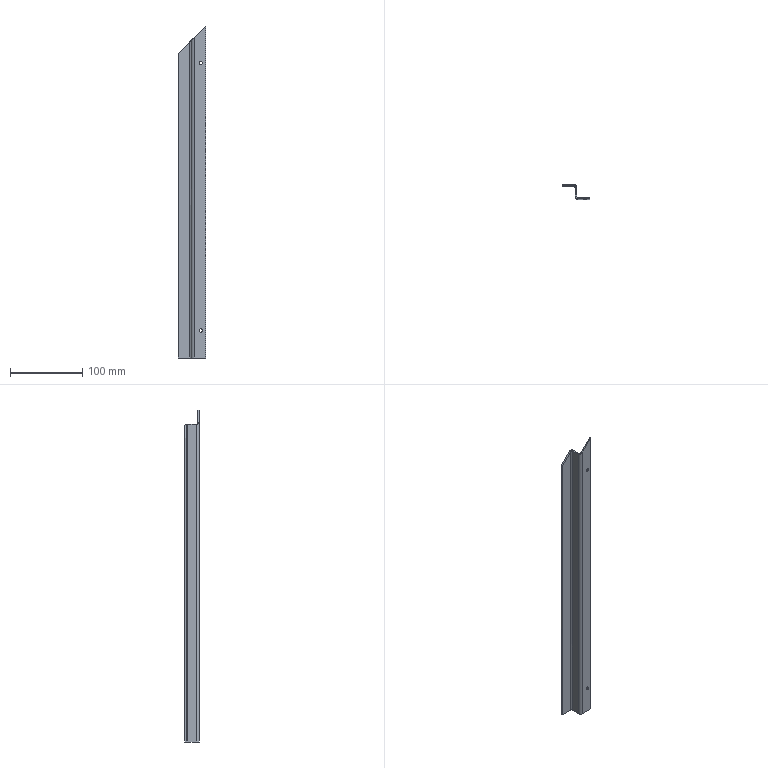Part | STEP file | SYL_0392D6J1SYL0380DJ10-1205588 | 1 solid | 26 faces | box 38 x 20 x 458 mm | volume 46808 mm3 | plane 16 | cylinder 8 | spline 2 | commonest cylinder face diameters 4.5 x4 4 x2 8 x2
STEP:
#1=CARTESIAN_POINT('',(11.,-20.,-193.25));
#2=VERTEX_POINT('',#1);
#3=CARTESIAN_POINT('',(11.,-18.,-193.25));
#4=VERTEX_POINT('',#3);
#5=CARTESIAN_POINT('',(11.,-18.,-193.25));
#6=DIRECTION('',(0.,1.,0.));
#7=VECTOR('',#6,1000.);
#8=LINE('',#5,#7);
#9=EDGE_CURVE('',#2,#4,#8,.T.);
#10=ORIENTED_EDGE('',*,*,#9,.F.);
#11=CARTESIAN_POINT('',(11.,-20.,-188.75));
#12=VERTEX_POINT('',#11);
#13=CARTESIAN_POINT('',(11.,-20.,-191.));
#14=DIRECTION('',(0.,-1.,0.));
#15=DIRECTION('',(0.,0.,-1.));
#16=AXIS2_PLACEMENT_3D('',#13,#14,#15);
#17=CIRCLE('',#16,2.25);
#18=EDGE_CURVE('',#2,#12,#17,.T.);
#19=ORIENTED_EDGE('',*,*,#18,.T.);
#20=CARTESIAN_POINT('',(11.,-18.,-188.75));
#21=VERTEX_POINT('',#20);
#22=CARTESIAN_POINT('',(11.,-18.,-188.75));
#23=DIRECTION('',(0.,1.,0.));
#24=VECTOR('',#23,1000.);
#25=LINE('',#22,#24);
#26=EDGE_CURVE('',#12,#21,#25,.T.);
#27=ORIENTED_EDGE('',*,*,#26,.T.);
#28=CARTESIAN_POINT('',(11.,-18.,-191.));
#29=DIRECTION('',(0.,-1.,0.));
#30=DIRECTION('',(0.,0.,-1.));
#31=AXIS2_PLACEMENT_3D('',#28,#29,#30);
#32=CIRCLE('',#31,2.25);
#33=EDGE_CURVE('',#4,#21,#32,.T.);
#34=ORIENTED_EDGE('',*,*,#33,.F.);
#35=EDGE_LOOP('',(#10,#19,#27,#34));
#36=FACE_OUTER_BOUND('',#35,.T.);
#37=CARTESIAN_POINT('',(11.,-18.,-191.));
#38=DIRECTION('',(0.,1.,0.));
#39=DIRECTION('',(0.,0.,1.));
#40=AXIS2_PLACEMENT_3D('',#37,#38,#39);
#41=CYLINDRICAL_SURFACE('',#40,2.25);
#42=ADVANCED_FACE('',(#36),#41,.F.);
#43=CARTESIAN_POINT('',(11.,-20.,175.75));
#44=VERTEX_POINT('',#43);
#45=CARTESIAN_POINT('',(11.,-18.,175.75));
#46=VERTEX_POINT('',#45);
#47=CARTESIAN_POINT('',(11.,-18.,175.75));
#48=DIRECTION('',(0.,1.,0.));
#49=VECTOR('',#48,1000.);
#50=LINE('',#47,#49);
#51=EDGE_CURVE('',#44,#46,#50,.T.);
#52=ORIENTED_EDGE('',*,*,#51,.F.);
#53=CARTESIAN_POINT('',(11.,-20.,180.25));
#54=VERTEX_POINT('',#53);
#55=CARTESIAN_POINT('',(11.,-20.,178.));
#56=DIRECTION('',(0.,-1.,0.));
#57=DIRECTION('',(0.,0.,-1.));
#58=AXIS2_PLACEMENT_3D('',#55,#56,#57);
#59=CIRCLE('',#58,2.25);
#60=EDGE_CURVE('',#44,#54,#59,.T.);
#61=ORIENTED_EDGE('',*,*,#60,.T.);
#62=CARTESIAN_POINT('',(11.,-18.,180.25));
#63=VERTEX_POINT('',#62);
#64=CARTESIAN_POINT('',(11.,-18.,180.25));
#65=DIRECTION('',(0.,1.,0.));
#66=VECTOR('',#65,1000.);
#67=LINE('',#64,#66);
#68=EDGE_CURVE('',#54,#63,#67,.T.);
#69=ORIENTED_EDGE('',*,*,#68,.T.);
#70=CARTESIAN_POINT('',(11.,-18.,178.));
#71=DIRECTION('',(0.,-1.,0.));
#72=DIRECTION('',(0.,0.,-1.));
#73=AXIS2_PLACEMENT_3D('',#70,#71,#72);
#74=CIRCLE('',#73,2.25);
#75=EDGE_CURVE('',#46,#63,#74,.T.);
#76=ORIENTED_EDGE('',*,*,#75,.F.);
#77=EDGE_LOOP('',(#52,#61,#69,#76));
#78=FACE_OUTER_BOUND('',#77,.T.);
#79=CARTESIAN_POINT('',(11.,-18.,178.));
#80=DIRECTION('',(0.,1.,0.));
#81=DIRECTION('',(0.,0.,1.));
#82=AXIS2_PLACEMENT_3D('',#79,#80,#81);
#83=CYLINDRICAL_SURFACE('',#82,2.25);
#84=ADVANCED_FACE('',(#78),#83,.F.);
#85=CARTESIAN_POINT('',(-2.,-16.,209.));
#86=VERTEX_POINT('',#85);
#87=CARTESIAN_POINT('',(0.,-16.,209.));
#88=VERTEX_POINT('',#87);
#89=CARTESIAN_POINT('',(-2.,-16.,209.));
#90=CARTESIAN_POINT('',(-1.333,-16.,209.));
#91=CARTESIAN_POINT('',(-0.6667,-16.,209.));
#92=CARTESIAN_POINT('',(0.,-16.,209.));
#93=B_SPLINE_CURVE_WITH_KNOTS('',3,(#89,#90,#91,#92),.UNSPECIFIED.,.F.,.F.,(4,4),(0.,1.),.UNSPECIFIED.);
#94=EDGE_CURVE('',#86,#88,#93,.T.);
#95=ORIENTED_EDGE('',*,*,#94,.F.);
#96=CARTESIAN_POINT('',(2.,-20.,213.));
#97=VERTEX_POINT('',#96);
#98=CARTESIAN_POINT('',(-2.,-16.,209.));
#99=CARTESIAN_POINT('',(-2.,-16.468,209.));
#100=CARTESIAN_POINT('',(-1.917,-16.94,209.083));
#101=CARTESIAN_POINT('',(-1.669,-17.61,209.331));
#102=CARTESIAN_POINT('',(-1.565,-17.831,209.435));
#103=CARTESIAN_POINT('',(-1.376,-18.15,209.625));
#104=CARTESIAN_POINT('',(-1.307,-18.254,209.693));
#105=CARTESIAN_POINT('',(-1.196,-18.406,209.804));
#106=CARTESIAN_POINT('',(-1.158,-18.456,209.843));
#107=CARTESIAN_POINT('',(-1.098,-18.531,209.902));
#108=CARTESIAN_POINT('',(-1.078,-18.555,209.922));
#109=CARTESIAN_POINT('',(-1.047,-18.592,209.953));
#110=CARTESIAN_POINT('',(-1.036,-18.604,209.964));
#111=CARTESIAN_POINT('',(-1.016,-18.628,209.984));
#112=CARTESIAN_POINT('',(-1.004,-18.641,209.996));
#113=CARTESIAN_POINT('',(-0.8372,-18.83,210.163));
#114=CARTESIAN_POINT('',(-0.6565,-19.002,210.344));
#115=CARTESIAN_POINT('',(-0.349,-19.24,210.652));
#116=CARTESIAN_POINT('',(-0.2404,-19.316,210.76));
#117=CARTESIAN_POINT('',(-0.06848,-19.424,210.932));
#118=CARTESIAN_POINT('',(-0.009675,-19.459,210.991));
#119=CARTESIAN_POINT('',(0.08075,-19.51,211.081));
#120=CARTESIAN_POINT('',(0.1113,-19.526,211.111));
#121=CARTESIAN_POINT('',(0.1576,-19.55,211.158));
#122=CARTESIAN_POINT('',(0.1731,-19.558,211.173));
#123=CARTESIAN_POINT('',(0.2043,-19.574,211.204));
#124=CARTESIAN_POINT('',(0.2213,-19.583,211.221));
#125=CARTESIAN_POINT('',(0.352,-19.647,211.352));
#126=CARTESIAN_POINT('',(0.4773,-19.702,211.477));
#127=CARTESIAN_POINT('',(0.6793,-19.776,211.679));
#128=CARTESIAN_POINT('',(0.749,-19.8,211.749));
#129=CARTESIAN_POINT('',(0.8569,-19.833,211.857));
#130=CARTESIAN_POINT('',(0.8935,-19.844,211.894));
#131=CARTESIAN_POINT('',(0.9492,-19.86,211.949));
#132=CARTESIAN_POINT('',(0.9679,-19.865,211.968));
#133=CARTESIAN_POINT('',(0.9962,-19.872,211.996));
#134=CARTESIAN_POINT('',(1.006,-19.874,212.006));
#135=CARTESIAN_POINT('',(1.02,-19.878,212.02));
#136=CARTESIAN_POINT('',(1.025,-19.879,212.025));
#137=CARTESIAN_POINT('',(1.034,-19.882,212.034));
#138=CARTESIAN_POINT('',(1.041,-19.883,212.041));
#139=CARTESIAN_POINT('',(1.252,-19.935,212.252));
#140=CARTESIAN_POINT('',(1.571,-20.,212.571));
#141=CARTESIAN_POINT('',(2.,-20.,213.));
#142=B_SPLINE_CURVE_WITH_KNOTS('',3,(#98,#99,#100,#101,#102,#103,#104,#105,#106,#107,#108,#109,#110,#111,#112,#113,#114,#115,#116,#117,#118,#119,#120,#121,#122,#123,#124,#125,#126,#127,#128,#129,#130,#131,#132,#133,#134,#135,#136,#137,#138,#139,#140,#141),.UNSPECIFIED.,.F.,.F.,(4,2,2,2,2,2,2,2,2,2,2,2,2,2,2,2,2,2,2,2,2,4),(0.,0.25,0.375,0.4375,0.4688,0.4844,0.4922,0.5,0.625,0.6875,0.7188,0.7344,0.7422,0.75,0.8125,0.8438,0.8594,0.8672,0.8711,0.873,0.875,1.),.UNSPECIFIED.);
#143=EDGE_CURVE('',#86,#97,#142,.T.);
#144=ORIENTED_EDGE('',*,*,#143,.T.);
#145=CARTESIAN_POINT('',(2.,-18.,213.));
#146=VERTEX_POINT('',#145);
#147=CARTESIAN_POINT('',(2.,-20.,213.));
#148=CARTESIAN_POINT('',(2.,-18.,213.));
#149=B_SPLINE_CURVE_WITH_KNOTS('',1,(#147,#148),.UNSPECIFIED.,.F.,.F.,(2,2),(0.,1.),.UNSPECIFIED.);
#150=EDGE_CURVE('',#97,#146,#149,.T.);
#151=ORIENTED_EDGE('',*,*,#150,.T.);
#152=CARTESIAN_POINT('',(0.,-16.,209.));
#153=CARTESIAN_POINT('',(0.,-16.234,209.));
#154=CARTESIAN_POINT('',(0.04143,-16.47,209.083));
#155=CARTESIAN_POINT('',(0.1654,-16.805,209.331));
#156=CARTESIAN_POINT('',(0.2175,-16.915,209.435));
#157=CARTESIAN_POINT('',(0.3122,-17.075,209.625));
#158=CARTESIAN_POINT('',(0.3465,-17.127,209.693));
#159=CARTESIAN_POINT('',(0.402,-17.203,209.804));
#160=CARTESIAN_POINT('',(0.4308,-17.241,209.862));
#161=CARTESIAN_POINT('',(0.4612,-17.278,209.922));
#162=CARTESIAN_POINT('',(0.4817,-17.302,209.963));
#163=CARTESIAN_POINT('',(0.4929,-17.315,209.986));
#164=CARTESIAN_POINT('',(0.5814,-17.415,210.163));
#165=CARTESIAN_POINT('',(0.6717,-17.501,210.344));
#166=CARTESIAN_POINT('',(0.8255,-17.62,210.652));
#167=CARTESIAN_POINT('',(0.8798,-17.658,210.76));
#168=CARTESIAN_POINT('',(0.9658,-17.712,210.932));
#169=CARTESIAN_POINT('',(1.01,-17.738,211.02));
#170=CARTESIAN_POINT('',(1.063,-17.767,211.127));
#171=CARTESIAN_POINT('',(1.087,-17.779,211.173));
#172=CARTESIAN_POINT('',(1.102,-17.787,211.204));
#173=CARTESIAN_POINT('',(1.111,-17.791,211.221));
#174=CARTESIAN_POINT('',(1.176,-17.824,211.352));
#175=CARTESIAN_POINT('',(1.239,-17.851,211.477));
#176=CARTESIAN_POINT('',(1.34,-17.888,211.679));
#177=CARTESIAN_POINT('',(1.374,-17.9,211.749));
#178=CARTESIAN_POINT('',(1.428,-17.917,211.857));
#179=CARTESIAN_POINT('',(1.456,-17.925,211.912));
#180=CARTESIAN_POINT('',(1.489,-17.934,211.977));
#181=CARTESIAN_POINT('',(1.505,-17.938,212.01));
#182=CARTESIAN_POINT('',(1.512,-17.94,212.025));
#183=CARTESIAN_POINT('',(1.517,-17.941,212.034));
#184=CARTESIAN_POINT('',(1.52,-17.942,212.041));
#185=CARTESIAN_POINT('',(1.626,-17.968,212.252));
#186=CARTESIAN_POINT('',(1.786,-18.,212.571));
#187=CARTESIAN_POINT('',(2.,-18.,213.));
#188=B_SPLINE_CURVE_WITH_KNOTS('',3,(#152,#153,#154,#155,#156,#157,#158,#159,#160,#161,#162,#163,#164,#165,#166,#167,#168,#169,#170,#171,#172,#173,#174,#175,#176,#177,#178,#179,#180,#181,#182,#183,#184,#185,#186,#187),.UNSPECIFIED.,.F.,.F.,(4,2,2,2,1,2,2,2,2,1,1,2,2,2,2,1,1,1,2,2,4),(0.,0.25,0.375,0.4375,0.4688,0.4844,0.5,0.625,0.6875,0.7188,0.7344,0.7422,0.75,0.8125,0.8438,0.8594,0.8672,0.8711,0.873,0.875,1.),.UNSPECIFIED.);
#189=EDGE_CURVE('',#88,#146,#188,.T.);
#190=ORIENTED_EDGE('',*,*,#189,.F.);
#191=EDGE_LOOP('',(#95,#144,#151,#190));
#192=FACE_OUTER_BOUND('',#191,.T.);
#193=CARTESIAN_POINT('',(-2.,-16.,209.));
#194=CARTESIAN_POINT('',(-2.,-16.468,209.));
#195=CARTESIAN_POINT('',(-1.917,-16.94,209.083));
#196=CARTESIAN_POINT('',(-1.669,-17.61,209.331));
#197=CARTESIAN_POINT('',(-1.565,-17.831,209.435));
#198=CARTESIAN_POINT('',(-1.376,-18.15,209.625));
#199=CARTESIAN_POINT('',(-1.307,-18.254,209.693));
#200=CARTESIAN_POINT('',(-1.196,-18.406,209.804));
#201=CARTESIAN_POINT('',(-1.158,-18.456,209.843));
#202=CARTESIAN_POINT('',(-1.098,-18.531,209.902));
#203=CARTESIAN_POINT('',(-1.078,-18.555,209.922));
#204=CARTESIAN_POINT('',(-1.047,-18.592,209.953));
#205=CARTESIAN_POINT('',(-1.036,-18.604,209.964));
#206=CARTESIAN_POINT('',(-1.016,-18.628,209.984));
#207=CARTESIAN_POINT('',(-1.004,-18.641,209.996));
#208=CARTESIAN_POINT('',(-0.8372,-18.83,210.163));
#209=CARTESIAN_POINT('',(-0.6565,-19.002,210.344));
#210=CARTESIAN_POINT('',(-0.349,-19.24,210.652));
#211=CARTESIAN_POINT('',(-0.2404,-19.316,210.76));
#212=CARTESIAN_POINT('',(-0.06848,-19.424,210.932));
#213=CARTESIAN_POINT('',(-0.009675,-19.459,210.991));
#214=CARTESIAN_POINT('',(0.08075,-19.51,211.081));
#215=CARTESIAN_POINT('',(0.1113,-19.526,211.111));
#216=CARTESIAN_POINT('',(0.1576,-19.55,211.158));
#217=CARTESIAN_POINT('',(0.1731,-19.558,211.173));
#218=CARTESIAN_POINT('',(0.2043,-19.574,211.204));
#219=CARTESIAN_POINT('',(0.2213,-19.583,211.221));
#220=CARTESIAN_POINT('',(0.352,-19.647,211.352));
#221=CARTESIAN_POINT('',(0.4773,-19.702,211.477));
#222=CARTESIAN_POINT('',(0.6793,-19.776,211.679));
#223=CARTESIAN_POINT('',(0.749,-19.8,211.749));
#224=CARTESIAN_POINT('',(0.8569,-19.833,211.857));
#225=CARTESIAN_POINT('',(0.8935,-19.844,211.894));
#226=CARTESIAN_POINT('',(0.9492,-19.86,211.949));
#227=CARTESIAN_POINT('',(0.9679,-19.865,211.968));
#228=CARTESIAN_POINT('',(0.9962,-19.872,211.996));
#229=CARTESIAN_POINT('',(1.006,-19.874,212.006));
#230=CARTESIAN_POINT('',(1.02,-19.878,212.02));
#231=CARTESIAN_POINT('',(1.025,-19.879,212.025));
#232=CARTESIAN_POINT('',(1.034,-19.882,212.034));
#233=CARTESIAN_POINT('',(1.041,-19.883,212.041));
#234=CARTESIAN_POINT('',(1.252,-19.935,212.252));
#235=CARTESIAN_POINT('',(1.571,-20.,212.571));
#236=CARTESIAN_POINT('',(2.,-20.,213.));
#237=CARTESIAN_POINT('',(0.,-16.,209.));
#238=CARTESIAN_POINT('',(0.,-16.234,209.));
#239=CARTESIAN_POINT('',(0.04143,-16.47,209.083));
#240=CARTESIAN_POINT('',(0.1654,-16.805,209.331));
#241=CARTESIAN_POINT('',(0.2175,-16.915,209.435));
#242=CARTESIAN_POINT('',(0.3122,-17.075,209.625));
#243=CARTESIAN_POINT('',(0.3465,-17.127,209.693));
#244=CARTESIAN_POINT('',(0.402,-17.203,209.804));
#245=CARTESIAN_POINT('',(0.4212,-17.228,209.843));
#246=CARTESIAN_POINT('',(0.4511,-17.265,209.902));
#247=CARTESIAN_POINT('',(0.4612,-17.278,209.922));
#248=CARTESIAN_POINT('',(0.4766,-17.296,209.953));
#249=CARTESIAN_POINT('',(0.4818,-17.302,209.964));
#250=CARTESIAN_POINT('',(0.4922,-17.314,209.984));
#251=CARTESIAN_POINT('',(0.4978,-17.32,209.996));
#252=CARTESIAN_POINT('',(0.5814,-17.415,210.163));
#253=CARTESIAN_POINT('',(0.6717,-17.501,210.344));
#254=CARTESIAN_POINT('',(0.8255,-17.62,210.652));
#255=CARTESIAN_POINT('',(0.8798,-17.658,210.76));
#256=CARTESIAN_POINT('',(0.9658,-17.712,210.932));
#257=CARTESIAN_POINT('',(0.9952,-17.73,210.991));
#258=CARTESIAN_POINT('',(1.04,-17.755,211.081));
#259=CARTESIAN_POINT('',(1.056,-17.763,211.111));
#260=CARTESIAN_POINT('',(1.079,-17.775,211.158));
#261=CARTESIAN_POINT('',(1.087,-17.779,211.173));
#262=CARTESIAN_POINT('',(1.102,-17.787,211.204));
#263=CARTESIAN_POINT('',(1.111,-17.791,211.221));
#264=CARTESIAN_POINT('',(1.176,-17.824,211.352));
#265=CARTESIAN_POINT('',(1.239,-17.851,211.477));
#266=CARTESIAN_POINT('',(1.34,-17.888,211.679));
#267=CARTESIAN_POINT('',(1.374,-17.9,211.749));
#268=CARTESIAN_POINT('',(1.428,-17.917,211.857));
#269=CARTESIAN_POINT('',(1.447,-17.922,211.894));
#270=CARTESIAN_POINT('',(1.475,-17.93,211.949));
#271=CARTESIAN_POINT('',(1.484,-17.932,211.968));
#272=CARTESIAN_POINT('',(1.498,-17.936,211.996));
#273=CARTESIAN_POINT('',(1.503,-17.937,212.006));
#274=CARTESIAN_POINT('',(1.51,-17.939,212.02));
#275=CARTESIAN_POINT('',(1.512,-17.94,212.025));
#276=CARTESIAN_POINT('',(1.517,-17.941,212.034));
#277=CARTESIAN_POINT('',(1.52,-17.942,212.041));
#278=CARTESIAN_POINT('',(1.626,-17.968,212.252));
#279=CARTESIAN_POINT('',(1.785,-18.,212.571));
#280=CARTESIAN_POINT('',(2.,-18.,213.));
#281=B_SPLINE_SURFACE_WITH_KNOTS('',1,3,((#193,#194,#195,#196,#197,#198,#199,#200,#201,#202,#203,#204,#205,#206,#207,#208,#209,#210,#211,#212,#213,#214,#215,#216,#217,#218,#219,#220,#221,#222,#223,#224,#225,#226,#227,#228,#229,#230,#231,#232,#233,#234,#235,#236),(#237,#238,#239,#240,#241,#242,#243,#244,#245,#246,#247,#248,#249,#250,#251,#252,#253,#254,#255,#256,#257,#258,#259,#260,#261,#262,#263,#264,#265,#266,#267,#268,#269,#270,#271,#272,#273,#274,#275,#276,#277,#278,#279,#280)),.UNSPECIFIED.,.F.,.F.,.F.,(2,2),(4,2,2,2,2,2,2,2,2,2,2,2,2,2,2,2,2,2,2,2,2,4),(0.,1.),(0.,0.25,0.375,0.4375,0.4688,0.4844,0.4922,0.5,0.625,0.6875,0.7188,0.7344,0.7422,0.75,0.8125,0.8438,0.8594,0.8672,0.8711,0.873,0.875,1.),.UNSPECIFIED.);
#282=ADVANCED_FACE('',(#192),#281,.F.);
#283=ORIENTED_EDGE('',*,*,#150,.F.);
#284=CARTESIAN_POINT('',(18.,-20.,229.));
#285=VERTEX_POINT('',#284);
#286=CARTESIAN_POINT('',(2.,-20.,213.));
#287=DIRECTION('',(0.7071,0.,0.7071));
#288=VECTOR('',#287,1000.);
#289=LINE('',#286,#288);
#290=EDGE_CURVE('',#97,#285,#289,.T.);
#291=ORIENTED_EDGE('',*,*,#290,.T.);
#292=CARTESIAN_POINT('',(18.,-18.,229.));
#293=VERTEX_POINT('',#292);
#294=CARTESIAN_POINT('',(18.,-18.,229.));
#295=DIRECTION('',(0.,1.,0.));
#296=VECTOR('',#295,1000.);
#297=LINE('',#294,#296);
#298=EDGE_CURVE('',#285,#293,#297,.T.);
#299=ORIENTED_EDGE('',*,*,#298,.T.);
#300=CARTESIAN_POINT('',(2.,-18.,213.));
#301=DIRECTION('',(0.7071,0.,0.7071));
#302=VECTOR('',#301,1000.);
#303=LINE('',#300,#302);
#304=EDGE_CURVE('',#146,#293,#303,.T.);
#305=ORIENTED_EDGE('',*,*,#304,.F.);
#306=EDGE_LOOP('',(#283,#291,#299,#305));
#307=FACE_OUTER_BOUND('',#306,.T.);
#308=CARTESIAN_POINT('',(2.,-18.,213.));
#309=DIRECTION('',(-0.7071,0.,0.7071));
#310=DIRECTION('',(0.7071,0.,0.7071));
#311=AXIS2_PLACEMENT_3D('',#308,#309,#310);
#312=PLANE('',#311);
#313=ADVANCED_FACE('',(#307),#312,.T.);
#314=ORIENTED_EDGE('',*,*,#298,.F.);
#315=CARTESIAN_POINT('',(18.,-20.,-229.));
#316=VERTEX_POINT('',#315);
#317=CARTESIAN_POINT('',(18.,-20.,-229.));
#318=DIRECTION('',(0.,0.,1.));
#319=VECTOR('',#318,1000.);
#320=LINE('',#317,#319);
#321=EDGE_CURVE('',#316,#285,#320,.T.);
#322=ORIENTED_EDGE('',*,*,#321,.F.);
#323=CARTESIAN_POINT('',(18.,-18.,-229.));
#324=VERTEX_POINT('',#323);
#325=CARTESIAN_POINT('',(18.,-18.,-229.));
#326=DIRECTION('',(0.,1.,0.));
#327=VECTOR('',#326,1000.);
#328=LINE('',#325,#327);
#329=EDGE_CURVE('',#316,#324,#328,.T.);
#330=ORIENTED_EDGE('',*,*,#329,.T.);
#331=CARTESIAN_POINT('',(18.,-18.,-229.));
#332=DIRECTION('',(0.,0.,1.));
#333=VECTOR('',#332,1000.);
#334=LINE('',#331,#333);
#335=EDGE_CURVE('',#324,#293,#334,.T.);
#336=ORIENTED_EDGE('',*,*,#335,.T.);
#337=EDGE_LOOP('',(#314,#322,#330,#336));
#338=FACE_OUTER_BOUND('',#337,.T.);
#339=CARTESIAN_POINT('',(18.,-18.,-229.));
#340=DIRECTION('',(-1.,0.,0.));
#341=DIRECTION('',(0.,0.,1.));
#342=AXIS2_PLACEMENT_3D('',#339,#340,#341);
#343=PLANE('',#342);
#344=ADVANCED_FACE('',(#338),#343,.F.);
#345=ORIENTED_EDGE('',*,*,#329,.F.);
#346=CARTESIAN_POINT('',(2.,-20.,-229.));
#347=VERTEX_POINT('',#346);
#348=CARTESIAN_POINT('',(18.,-20.,-229.));
#349=DIRECTION('',(-1.,0.,0.));
#350=VECTOR('',#349,1000.);
#351=LINE('',#348,#350);
#352=EDGE_CURVE('',#316,#347,#351,.T.);
#353=ORIENTED_EDGE('',*,*,#352,.T.);
#354=CARTESIAN_POINT('',(2.,-18.,-229.));
#355=VERTEX_POINT('',#354);
#356=CARTESIAN_POINT('',(2.,-18.,-229.));
#357=DIRECTION('',(0.,1.,0.));
#358=VECTOR('',#357,1000.);
#359=LINE('',#356,#358);
#360=EDGE_CURVE('',#347,#355,#359,.T.);
#361=ORIENTED_EDGE('',*,*,#360,.T.);
#362=CARTESIAN_POINT('',(18.,-18.,-229.));
#363=DIRECTION('',(-1.,0.,0.));
#364=VECTOR('',#363,1000.);
#365=LINE('',#362,#364);
#366=EDGE_CURVE('',#324,#355,#365,.T.);
#367=ORIENTED_EDGE('',*,*,#366,.F.);
#368=EDGE_LOOP('',(#345,#353,#361,#367));
#369=FACE_OUTER_BOUND('',#368,.T.);
#370=CARTESIAN_POINT('',(18.,-18.,-229.));
#371=DIRECTION('',(0.,0.,-1.));
#372=DIRECTION('',(-1.,0.,0.));
#373=AXIS2_PLACEMENT_3D('',#370,#371,#372);
#374=PLANE('',#373);
#375=ADVANCED_FACE('',(#369),#374,.T.);
#376=ORIENTED_EDGE('',*,*,#360,.F.);
#377=CARTESIAN_POINT('',(-2.,-16.,-229.));
#378=VERTEX_POINT('',#377);
#379=CARTESIAN_POINT('',(2.,-16.,-229.));
#380=DIRECTION('',(0.,0.,1.));
#381=DIRECTION('',(1.,0.,0.));
#382=AXIS2_PLACEMENT_3D('',#379,#380,#381);
#383=CIRCLE('',#382,4.);
#384=EDGE_CURVE('',#378,#347,#383,.T.);
#385=ORIENTED_EDGE('',*,*,#384,.F.);
#386=CARTESIAN_POINT('',(0.,-16.,-229.));
#387=VERTEX_POINT('',#386);
#388=CARTESIAN_POINT('',(0.,-16.,-229.));
#389=DIRECTION('',(1.,0.,0.));
#390=VECTOR('',#389,1000.);
#391=LINE('',#388,#390);
#392=EDGE_CURVE('',#378,#387,#391,.T.);
#393=ORIENTED_EDGE('',*,*,#392,.T.);
#394=CARTESIAN_POINT('',(2.,-16.,-229.));
#395=DIRECTION('',(0.,0.,1.));
#396=DIRECTION('',(-1.,0.,0.));
#397=AXIS2_PLACEMENT_3D('',#394,#395,#396);
#398=CIRCLE('',#397,2.);
#399=EDGE_CURVE('',#387,#355,#398,.T.);
#400=ORIENTED_EDGE('',*,*,#399,.T.);
#401=EDGE_LOOP('',(#376,#385,#393,#400));
#402=FACE_OUTER_BOUND('',#401,.T.);
#403=CARTESIAN_POINT('',(2.,-16.,-229.));
#404=DIRECTION('',(0.,0.,-1.));
#405=DIRECTION('',(-1.,0.,0.));
#406=AXIS2_PLACEMENT_3D('',#403,#404,#405);
#407=PLANE('',#406);
#408=ADVANCED_FACE('',(#402),#407,.T.);
#409=ORIENTED_EDGE('',*,*,#392,.F.);
#410=CARTESIAN_POINT('',(-2.,-4.,-229.));
#411=VERTEX_POINT('',#410);
#412=CARTESIAN_POINT('',(-2.,-16.,-229.));
#413=DIRECTION('',(0.,1.,0.));
#414=VECTOR('',#413,1000.);
#415=LINE('',#412,#414);
#416=EDGE_CURVE('',#378,#411,#415,.T.);
#417=ORIENTED_EDGE('',*,*,#416,.T.);
#418=CARTESIAN_POINT('',(0.,-4.,-229.));
#419=VERTEX_POINT('',#418);
#420=CARTESIAN_POINT('',(0.,-4.,-229.));
#421=DIRECTION('',(1.,0.,0.));
#422=VECTOR('',#421,1000.);
#423=LINE('',#420,#422);
#424=EDGE_CURVE('',#411,#419,#423,.T.);
#425=ORIENTED_EDGE('',*,*,#424,.T.);
#426=CARTESIAN_POINT('',(0.,-16.,-229.));
#427=DIRECTION('',(0.,1.,0.));
#428=VECTOR('',#427,1000.);
#429=LINE('',#426,#428);
#430=EDGE_CURVE('',#387,#419,#429,.T.);
#431=ORIENTED_EDGE('',*,*,#430,.F.);
#432=EDGE_LOOP('',(#409,#417,#425,#431));
#433=FACE_OUTER_BOUND('',#432,.T.);
#434=CARTESIAN_POINT('',(0.,-16.,-229.));
#435=DIRECTION('',(0.,0.,-1.));
#436=DIRECTION('',(0.,1.,0.));
#437=AXIS2_PLACEMENT_3D('',#434,#435,#436);
#438=PLANE('',#437);
#439=ADVANCED_FACE('',(#433),#438,.T.);
#440=ORIENTED_EDGE('',*,*,#424,.F.);
#441=CARTESIAN_POINT('',(-4.,-2.,-229.));
#442=VERTEX_POINT('',#441);
#443=CARTESIAN_POINT('',(-4.,-4.,-229.));
#444=DIRECTION('',(0.,0.,-1.));
#445=DIRECTION('',(1.,0.,0.));
#446=AXIS2_PLACEMENT_3D('',#443,#444,#445);
#447=CIRCLE('',#446,2.);
#448=EDGE_CURVE('',#442,#411,#447,.T.);
#449=ORIENTED_EDGE('',*,*,#448,.F.);
#450=CARTESIAN_POINT('',(-4.,0.,-229.));
#451=VERTEX_POINT('',#450);
#452=CARTESIAN_POINT('',(-4.,0.,-229.));
#453=DIRECTION('',(0.,1.,0.));
#454=VECTOR('',#453,1000.);
#455=LINE('',#452,#454);
#456=EDGE_CURVE('',#442,#451,#455,.T.);
#457=ORIENTED_EDGE('',*,*,#456,.T.);
#458=CARTESIAN_POINT('',(-4.,-4.,-229.));
#459=DIRECTION('',(0.,0.,-1.));
#460=DIRECTION('',(0.,1.,0.));
#461=AXIS2_PLACEMENT_3D('',#458,#459,#460);
#462=CIRCLE('',#461,4.);
#463=EDGE_CURVE('',#451,#419,#462,.T.);
#464=ORIENTED_EDGE('',*,*,#463,.T.);
#465=EDGE_LOOP('',(#440,#449,#457,#464));
#466=FACE_OUTER_BOUND('',#465,.T.);
#467=CARTESIAN_POINT('',(-4.,-4.,-229.));
#468=DIRECTION('',(0.,0.,1.));
#469=DIRECTION('',(1.,0.,0.));
#470=AXIS2_PLACEMENT_3D('',#467,#468,#469);
#471=PLANE('',#470);
#472=ADVANCED_FACE('',(#466),#471,.F.);
#473=ORIENTED_EDGE('',*,*,#456,.F.);
#474=CARTESIAN_POINT('',(-20.,-2.,-229.));
#475=VERTEX_POINT('',#474);
#476=CARTESIAN_POINT('',(-4.,-2.,-229.));
#477=DIRECTION('',(-1.,0.,0.));
#478=VECTOR('',#477,1000.);
#479=LINE('',#476,#478);
#480=EDGE_CURVE('',#442,#475,#479,.T.);
#481=ORIENTED_EDGE('',*,*,#480,.T.);
#482=CARTESIAN_POINT('',(-20.,0.,-229.));
#483=VERTEX_POINT('',#482);
#484=CARTESIAN_POINT('',(-20.,0.,-229.));
#485=DIRECTION('',(0.,1.,0.));
#486=VECTOR('',#485,1000.);
#487=LINE('',#484,#486);
#488=EDGE_CURVE('',#475,#483,#487,.T.);
#489=ORIENTED_EDGE('',*,*,#488,.T.);
#490=CARTESIAN_POINT('',(-4.,0.,-229.));
#491=DIRECTION('',(-1.,0.,0.));
#492=VECTOR('',#491,1000.);
#493=LINE('',#490,#492);
#494=EDGE_CURVE('',#451,#483,#493,.T.);
#495=ORIENTED_EDGE('',*,*,#494,.F.);
#496=EDGE_LOOP('',(#473,#481,#489,#495));
#497=FACE_OUTER_BOUND('',#496,.T.);
#498=CARTESIAN_POINT('',(-4.,0.,-229.));
#499=DIRECTION('',(0.,0.,-1.));
#500=DIRECTION('',(-1.,0.,0.));
#501=AXIS2_PLACEMENT_3D('',#498,#499,#500);
#502=PLANE('',#501);
#503=ADVANCED_FACE('',(#497),#502,.T.);
#504=ORIENTED_EDGE('',*,*,#488,.F.);
#505=CARTESIAN_POINT('',(-20.,-2.,191.));
#506=VERTEX_POINT('',#505);
#507=CARTESIAN_POINT('',(-20.,-2.,-229.));
#508=DIRECTION('',(0.,0.,1.));
#509=VECTOR('',#508,1000.);
#510=LINE('',#507,#509);
#511=EDGE_CURVE('',#475,#506,#510,.T.);
#512=ORIENTED_EDGE('',*,*,#511,.T.);
#513=CARTESIAN_POINT('',(-20.,0.,191.));
#514=VERTEX_POINT('',#513);
#515=CARTESIAN_POINT('',(-20.,0.,191.));
#516=DIRECTION('',(0.,1.,0.));
#517=VECTOR('',#516,1000.);
#518=LINE('',#515,#517);
#519=EDGE_CURVE('',#506,#514,#518,.T.);
#520=ORIENTED_EDGE('',*,*,#519,.T.);
#521=CARTESIAN_POINT('',(-20.,0.,-229.));
#522=DIRECTION('',(0.,0.,1.));
#523=VECTOR('',#522,1000.);
#524=LINE('',#521,#523);
#525=EDGE_CURVE('',#483,#514,#524,.T.);
#526=ORIENTED_EDGE('',*,*,#525,.F.);
#527=EDGE_LOOP('',(#504,#512,#520,#526));
#528=FACE_OUTER_BOUND('',#527,.T.);
#529=CARTESIAN_POINT('',(-20.,0.,-229.));
#530=DIRECTION('',(-1.,0.,0.));
#531=DIRECTION('',(0.,0.,1.));
#532=AXIS2_PLACEMENT_3D('',#529,#530,#531);
#533=PLANE('',#532);
#534=ADVANCED_FACE('',(#528),#533,.T.);
#535=ORIENTED_EDGE('',*,*,#519,.F.);
#536=CARTESIAN_POINT('',(-4.,-2.,207.));
#537=VERTEX_POINT('',#536);
#538=CARTESIAN_POINT('',(-20.,-2.,191.));
#539=DIRECTION('',(0.7071,0.,0.7071));
#540=VECTOR('',#539,1000.);
#541=LINE('',#538,#540);
#542=EDGE_CURVE('',#506,#537,#541,.T.);
#543=ORIENTED_EDGE('',*,*,#542,.T.);
#544=CARTESIAN_POINT('',(-4.,0.,207.));
#545=VERTEX_POINT('',#544);
#546=CARTESIAN_POINT('',(-4.,-2.,207.));
#547=CARTESIAN_POINT('',(-4.,-1.333,207.));
#548=CARTESIAN_POINT('',(-4.,-0.6667,207.));
#549=CARTESIAN_POINT('',(-4.,0.,207.));
#550=B_SPLINE_CURVE_WITH_KNOTS('',3,(#546,#547,#548,#549),.UNSPECIFIED.,.F.,.F.,(4,4),(0.,1.),.UNSPECIFIED.);
#551=EDGE_CURVE('',#537,#545,#550,.T.);
#552=ORIENTED_EDGE('',*,*,#551,.T.);
#553=CARTESIAN_POINT('',(-20.,0.,191.));
#554=DIRECTION('',(0.7071,0.,0.7071));
#555=VECTOR('',#554,1000.);
#556=LINE('',#553,#555);
#557=EDGE_CURVE('',#514,#545,#556,.T.);
#558=ORIENTED_EDGE('',*,*,#557,.F.);
#559=EDGE_LOOP('',(#535,#543,#552,#558));
#560=FACE_OUTER_BOUND('',#559,.T.);
#561=CARTESIAN_POINT('',(-20.,0.,191.));
#562=DIRECTION('',(-0.7071,0.,0.7071));
#563=DIRECTION('',(0.7071,0.,0.7071));
#564=AXIS2_PLACEMENT_3D('',#561,#562,#563);
#565=PLANE('',#564);
#566=ADVANCED_FACE('',(#560),#565,.T.);
#567=ORIENTED_EDGE('',*,*,#551,.F.);
#568=CARTESIAN_POINT('',(-2.,-4.,209.));
#569=VERTEX_POINT('',#568);
#570=CARTESIAN_POINT('',(-4.,-2.,207.));
#571=CARTESIAN_POINT('',(-3.837,-2.,207.163));
#572=CARTESIAN_POINT('',(-3.697,-2.02,207.302));
#573=CARTESIAN_POINT('',(-3.524,-2.057,207.476));
#574=CARTESIAN_POINT('',(-3.472,-2.07,207.528));
#575=CARTESIAN_POINT('',(-3.42,-2.086,207.58));
#576=CARTESIAN_POINT('',(-3.414,-2.088,207.585));
#577=CARTESIAN_POINT('',(-3.406,-2.09,207.594));
#578=CARTESIAN_POINT('',(-3.403,-2.091,207.596));
#579=CARTESIAN_POINT('',(-3.398,-2.093,207.602));
#580=CARTESIAN_POINT('',(-3.393,-2.094,207.607));
#581=CARTESIAN_POINT('',(-3.372,-2.101,207.628));
#582=CARTESIAN_POINT('',(-3.355,-2.107,207.645));
#583=CARTESIAN_POINT('',(-3.305,-2.124,207.694));
#584=CARTESIAN_POINT('',(-3.273,-2.137,207.727));
#585=CARTESIAN_POINT('',(-3.114,-2.202,207.885));
#586=CARTESIAN_POINT('',(-2.998,-2.265,208.001));
#587=CARTESIAN_POINT('',(-2.842,-2.368,208.157));
#588=CARTESIAN_POINT('',(-2.792,-2.405,208.206));
#589=CARTESIAN_POINT('',(-2.723,-2.461,208.276));
#590=CARTESIAN_POINT('',(-2.7,-2.479,208.298));
#591=CARTESIAN_POINT('',(-2.668,-2.508,208.331));
#592=CARTESIAN_POINT('',(-2.657,-2.518,208.342));
#593=CARTESIAN_POINT('',(-2.641,-2.532,208.358));
#594=CARTESIAN_POINT('',(-2.636,-2.537,208.363));
#595=CARTESIAN_POINT('',(-2.628,-2.545,208.371));
#596=CARTESIAN_POINT('',(-2.626,-2.547,208.373));
#597=CARTESIAN_POINT('',(-2.621,-2.552,208.378));
#598=CARTESIAN_POINT('',(-2.619,-2.554,208.38));
#599=CARTESIAN_POINT('',(-2.41,-2.754,208.589));
#600=CARTESIAN_POINT('',(-2.253,-2.989,208.743));
#601=CARTESIAN_POINT('',(-2.049,-3.486,208.949));
#602=CARTESIAN_POINT('',(-2.,-3.747,209.));
#603=CARTESIAN_POINT('',(-2.,-4.,209.));
#604=B_SPLINE_CURVE_WITH_KNOTS('',3,(#570,#571,#572,#573,#574,#575,#576,#577,#578,#579,#580,#581,#582,#583,#584,#585,#586,#587,#588,#589,#590,#591,#592,#593,#594,#595,#596,#597,#598,#599,#600,#601,#602,#603),.UNSPECIFIED.,.F.,.F.,(4,2,2,2,2,2,2,2,2,2,2,2,2,2,2,2,4),(0.,0.125,0.1875,0.1953,0.1992,0.2031,0.2188,0.25,0.375,0.4375,0.4688,0.4844,0.4922,0.4961,0.5,0.75,1.),.UNSPECIFIED.);
#605=EDGE_CURVE('',#537,#569,#604,.T.);
#606=ORIENTED_EDGE('',*,*,#605,.T.);
#607=CARTESIAN_POINT('',(0.,-4.,209.));
#608=VERTEX_POINT('',#607);
#609=CARTESIAN_POINT('',(-2.,-4.,209.));
#610=CARTESIAN_POINT('',(0.,-4.,209.));
#611=B_SPLINE_CURVE_WITH_KNOTS('',1,(#609,#610),.UNSPECIFIED.,.F.,.F.,(2,2),(0.,1.),.UNSPECIFIED.);
#612=EDGE_CURVE('',#569,#608,#611,.T.);
#613=ORIENTED_EDGE('',*,*,#612,.T.);
#614=CARTESIAN_POINT('',(-4.,0.,207.));
#615=CARTESIAN_POINT('',(-3.675,0.,207.163));
#616=CARTESIAN_POINT('',(-3.394,-0.03903,207.302));
#617=CARTESIAN_POINT('',(-3.047,-0.1133,207.476));
#618=CARTESIAN_POINT('',(-2.944,-0.1408,207.528));
#619=CARTESIAN_POINT('',(-2.84,-0.1719,207.58));
#620=CARTESIAN_POINT('',(-2.823,-0.177,207.588));
#621=CARTESIAN_POINT('',(-2.806,-0.1822,207.596));
#622=CARTESIAN_POINT('',(-2.796,-0.1857,207.602));
#623=CARTESIAN_POINT('',(-2.786,-0.1887,207.607));
#624=CARTESIAN_POINT('',(-2.744,-0.2023,207.628));
#625=CARTESIAN_POINT('',(-2.643,-0.236,207.678));
#626=CARTESIAN_POINT('',(-2.546,-0.2731,207.727));
#627=CARTESIAN_POINT('',(-2.228,-0.4034,207.885));
#628=CARTESIAN_POINT('',(-1.996,-0.5291,208.001));
#629=CARTESIAN_POINT('',(-1.683,-0.7367,208.157));
#630=CARTESIAN_POINT('',(-1.585,-0.8091,208.206));
#631=CARTESIAN_POINT('',(-1.446,-0.9211,208.276));
#632=CARTESIAN_POINT('',(-1.378,-0.9779,208.31));
#633=CARTESIAN_POINT('',(-1.303,-1.045,208.347));
#634=CARTESIAN_POINT('',(-1.267,-1.079,208.365));
#635=CARTESIAN_POINT('',(-1.251,-1.094,208.373));
#636=CARTESIAN_POINT('',(-1.241,-1.104,208.378));
#637=CARTESIAN_POINT('',(-1.237,-1.107,208.38));
#638=CARTESIAN_POINT('',(-0.82,-1.508,208.589));
#639=CARTESIAN_POINT('',(-0.5069,-1.978,208.743));
#640=CARTESIAN_POINT('',(-0.09717,-2.972,208.949));
#641=CARTESIAN_POINT('',(0.,-3.494,209.));
#642=CARTESIAN_POINT('',(0.,-4.,209.));
#643=B_SPLINE_CURVE_WITH_KNOTS('',3,(#614,#615,#616,#617,#618,#619,#620,#621,#622,#623,#624,#625,#626,#627,#628,#629,#630,#631,#632,#633,#634,#635,#636,#637,#638,#639,#640,#641,#642),.UNSPECIFIED.,.F.,.F.,(4,2,2,1,2,2,1,2,2,2,1,1,1,2,2,2,4),(0.,0.125,0.1875,0.1953,0.1992,0.2031,0.2188,0.25,0.375,0.4375,0.4687,0.4844,0.4922,0.4961,0.5,0.75,1.),.UNSPECIFIED.);
#644=EDGE_CURVE('',#545,#608,#643,.T.);
#645=ORIENTED_EDGE('',*,*,#644,.F.);
#646=EDGE_LOOP('',(#567,#606,#613,#645));
#647=FACE_OUTER_BOUND('',#646,.T.);
#648=CARTESIAN_POINT('',(-4.,0.,207.));
#649=CARTESIAN_POINT('',(-3.674,0.,207.163));
#650=CARTESIAN_POINT('',(-3.394,-0.03903,207.302));
#651=CARTESIAN_POINT('',(-3.047,-0.1133,207.476));
#652=CARTESIAN_POINT('',(-2.944,-0.1408,207.528));
#653=CARTESIAN_POINT('',(-2.84,-0.1719,207.58));
#654=CARTESIAN_POINT('',(-2.829,-0.1753,207.585));
#655=CARTESIAN_POINT('',(-2.812,-0.1805,207.594));
#656=CARTESIAN_POINT('',(-2.806,-0.1822,207.596));
#657=CARTESIAN_POINT('',(-2.796,-0.1857,207.602));
#658=CARTESIAN_POINT('',(-2.786,-0.1887,207.607));
#659=CARTESIAN_POINT('',(-2.744,-0.2023,207.628));
#660=CARTESIAN_POINT('',(-2.71,-0.2135,207.645));
#661=CARTESIAN_POINT('',(-2.611,-0.2483,207.694));
#662=CARTESIAN_POINT('',(-2.546,-0.2731,207.727));
#663=CARTESIAN_POINT('',(-2.228,-0.4034,207.885));
#664=CARTESIAN_POINT('',(-1.996,-0.5291,208.001));
#665=CARTESIAN_POINT('',(-1.683,-0.7367,208.157));
#666=CARTESIAN_POINT('',(-1.585,-0.8091,208.206));
#667=CARTESIAN_POINT('',(-1.446,-0.9211,208.276));
#668=CARTESIAN_POINT('',(-1.401,-0.959,208.298));
#669=CARTESIAN_POINT('',(-1.336,-1.016,208.331));
#670=CARTESIAN_POINT('',(-1.314,-1.036,208.342));
#671=CARTESIAN_POINT('',(-1.283,-1.065,208.358));
#672=CARTESIAN_POINT('',(-1.272,-1.074,208.363));
#673=CARTESIAN_POINT('',(-1.257,-1.089,208.371));
#674=CARTESIAN_POINT('',(-1.251,-1.094,208.373));
#675=CARTESIAN_POINT('',(-1.241,-1.104,208.378));
#676=CARTESIAN_POINT('',(-1.237,-1.107,208.38));
#677=CARTESIAN_POINT('',(-0.82,-1.508,208.589));
#678=CARTESIAN_POINT('',(-0.5069,-1.978,208.743));
#679=CARTESIAN_POINT('',(-0.09717,-2.972,208.949));
#680=CARTESIAN_POINT('',(0.,-3.495,209.));
#681=CARTESIAN_POINT('',(0.,-4.,209.));
#682=CARTESIAN_POINT('',(-4.,-2.,207.));
#683=CARTESIAN_POINT('',(-3.837,-2.,207.163));
#684=CARTESIAN_POINT('',(-3.697,-2.02,207.302));
#685=CARTESIAN_POINT('',(-3.524,-2.057,207.476));
#686=CARTESIAN_POINT('',(-3.472,-2.07,207.528));
#687=CARTESIAN_POINT('',(-3.42,-2.086,207.58));
#688=CARTESIAN_POINT('',(-3.414,-2.088,207.585));
#689=CARTESIAN_POINT('',(-3.406,-2.09,207.594));
#690=CARTESIAN_POINT('',(-3.403,-2.091,207.596));
#691=CARTESIAN_POINT('',(-3.398,-2.093,207.602));
#692=CARTESIAN_POINT('',(-3.393,-2.094,207.607));
#693=CARTESIAN_POINT('',(-3.372,-2.101,207.628));
#694=CARTESIAN_POINT('',(-3.355,-2.107,207.645));
#695=CARTESIAN_POINT('',(-3.305,-2.124,207.694));
#696=CARTESIAN_POINT('',(-3.273,-2.137,207.727));
#697=CARTESIAN_POINT('',(-3.114,-2.202,207.885));
#698=CARTESIAN_POINT('',(-2.998,-2.265,208.001));
#699=CARTESIAN_POINT('',(-2.842,-2.368,208.157));
#700=CARTESIAN_POINT('',(-2.792,-2.405,208.206));
#701=CARTESIAN_POINT('',(-2.723,-2.461,208.276));
#702=CARTESIAN_POINT('',(-2.7,-2.479,208.298));
#703=CARTESIAN_POINT('',(-2.668,-2.508,208.331));
#704=CARTESIAN_POINT('',(-2.657,-2.518,208.342));
#705=CARTESIAN_POINT('',(-2.641,-2.532,208.358));
#706=CARTESIAN_POINT('',(-2.636,-2.537,208.363));
#707=CARTESIAN_POINT('',(-2.628,-2.545,208.371));
#708=CARTESIAN_POINT('',(-2.626,-2.547,208.373));
#709=CARTESIAN_POINT('',(-2.621,-2.552,208.378));
#710=CARTESIAN_POINT('',(-2.619,-2.554,208.38));
#711=CARTESIAN_POINT('',(-2.41,-2.754,208.589));
#712=CARTESIAN_POINT('',(-2.253,-2.989,208.743));
#713=CARTESIAN_POINT('',(-2.049,-3.486,208.949));
#714=CARTESIAN_POINT('',(-2.,-3.747,209.));
#715=CARTESIAN_POINT('',(-2.,-4.,209.));
#716=B_SPLINE_SURFACE_WITH_KNOTS('',1,3,((#648,#649,#650,#651,#652,#653,#654,#655,#656,#657,#658,#659,#660,#661,#662,#663,#664,#665,#666,#667,#668,#669,#670,#671,#672,#673,#674,#675,#676,#677,#678,#679,#680,#681),(#682,#683,#684,#685,#686,#687,#688,#689,#690,#691,#692,#693,#694,#695,#696,#697,#698,#699,#700,#701,#702,#703,#704,#705,#706,#707,#708,#709,#710,#711,#712,#713,#714,#715)),.UNSPECIFIED.,.F.,.F.,.F.,(2,2),(4,2,2,2,2,2,2,2,2,2,2,2,2,2,2,2,4),(0.,1.),(0.,0.125,0.1875,0.1953,0.1992,0.2031,0.2188,0.25,0.375,0.4375,0.4688,0.4844,0.4922,0.4961,0.5,0.75,1.),.UNSPECIFIED.);
#717=ADVANCED_FACE('',(#647),#716,.T.);
#718=CARTESIAN_POINT('',(11.,-20.,178.));
#719=DIRECTION('',(0.,-1.,0.));
#720=DIRECTION('',(0.,0.,-1.));
#721=AXIS2_PLACEMENT_3D('',#718,#719,#720);
#722=CIRCLE('',#721,2.25);
#723=EDGE_CURVE('',#54,#44,#722,.T.);
#724=ORIENTED_EDGE('',*,*,#723,.T.);
#725=ORIENTED_EDGE('',*,*,#51,.T.);
#726=CARTESIAN_POINT('',(11.,-18.,178.));
#727=DIRECTION('',(0.,-1.,0.));
#728=DIRECTION('',(0.,0.,1.));
#729=AXIS2_PLACEMENT_3D('',#726,#727,#728);
#730=CIRCLE('',#729,2.25);
#731=EDGE_CURVE('',#63,#46,#730,.T.);
#732=ORIENTED_EDGE('',*,*,#731,.F.);
#733=ORIENTED_EDGE('',*,*,#68,.F.);
#734=EDGE_LOOP('',(#724,#725,#732,#733));
#735=FACE_OUTER_BOUND('',#734,.T.);
#736=CARTESIAN_POINT('',(11.,-18.,178.));
#737=DIRECTION('',(0.,1.,0.));
#738=DIRECTION('',(0.,0.,1.));
#739=AXIS2_PLACEMENT_3D('',#736,#737,#738);
#740=CYLINDRICAL_SURFACE('',#739,2.25);
#741=ADVANCED_FACE('',(#735),#740,.F.);
#742=CARTESIAN_POINT('',(11.,-20.,-191.));
#743=DIRECTION('',(0.,-1.,0.));
#744=DIRECTION('',(0.,0.,-1.));
#745=AXIS2_PLACEMENT_3D('',#742,#743,#744);
#746=CIRCLE('',#745,2.25);
#747=EDGE_CURVE('',#12,#2,#746,.T.);
#748=ORIENTED_EDGE('',*,*,#747,.T.);
#749=ORIENTED_EDGE('',*,*,#9,.T.);
#750=CARTESIAN_POINT('',(11.,-18.,-191.));
#751=DIRECTION('',(0.,-1.,0.));
#752=DIRECTION('',(0.,0.,1.));
#753=AXIS2_PLACEMENT_3D('',#750,#751,#752);
#754=CIRCLE('',#753,2.25);
#755=EDGE_CURVE('',#21,#4,#754,.T.);
#756=ORIENTED_EDGE('',*,*,#755,.F.);
#757=ORIENTED_EDGE('',*,*,#26,.F.);
#758=EDGE_LOOP('',(#748,#749,#756,#757));
#759=FACE_OUTER_BOUND('',#758,.T.);
#760=CARTESIAN_POINT('',(11.,-18.,-191.));
#761=DIRECTION('',(0.,1.,0.));
#762=DIRECTION('',(0.,0.,1.));
#763=AXIS2_PLACEMENT_3D('',#760,#761,#762);
#764=CYLINDRICAL_SURFACE('',#763,2.25);
#765=ADVANCED_FACE('',(#759),#764,.F.);
#766=CARTESIAN_POINT('',(-2.,-16.,209.));
#767=DIRECTION('',(0.,-1.,0.));
#768=VECTOR('',#767,1000.);
#769=LINE('',#766,#768);
#770=EDGE_CURVE('',#569,#86,#769,.T.);
#771=ORIENTED_EDGE('',*,*,#770,.T.);
#772=ORIENTED_EDGE('',*,*,#94,.T.);
#773=CARTESIAN_POINT('',(0.,-4.,209.));
#774=DIRECTION('',(0.,-1.,0.));
#775=VECTOR('',#774,1000.);
#776=LINE('',#773,#775);
#777=EDGE_CURVE('',#608,#88,#776,.T.);
#778=ORIENTED_EDGE('',*,*,#777,.F.);
#779=ORIENTED_EDGE('',*,*,#612,.F.);
#780=EDGE_LOOP('',(#771,#772,#778,#779));
#781=FACE_OUTER_BOUND('',#780,.T.);
#782=CARTESIAN_POINT('',(0.,-4.,209.));
#783=DIRECTION('',(0.,0.,1.));
#784=DIRECTION('',(0.,-1.,0.));
#785=AXIS2_PLACEMENT_3D('',#782,#783,#784);
#786=PLANE('',#785);
#787=ADVANCED_FACE('',(#781),#786,.T.);
#788=ORIENTED_EDGE('',*,*,#644,.T.);
#789=CARTESIAN_POINT('',(0.,-4.,209.));
#790=DIRECTION('',(0.,0.,-1.));
#791=VECTOR('',#790,1000.);
#792=LINE('',#789,#791);
#793=EDGE_CURVE('',#608,#419,#792,.T.);
#794=ORIENTED_EDGE('',*,*,#793,.T.);
#795=ORIENTED_EDGE('',*,*,#463,.F.);
#796=CARTESIAN_POINT('',(-4.,0.,-229.));
#797=DIRECTION('',(0.,0.,1.));
#798=VECTOR('',#797,1000.);
#799=LINE('',#796,#798);
#800=EDGE_CURVE('',#451,#545,#799,.T.);
#801=ORIENTED_EDGE('',*,*,#800,.T.);
#802=EDGE_LOOP('',(#788,#794,#795,#801));
#803=FACE_OUTER_BOUND('',#802,.T.);
#804=CARTESIAN_POINT('',(-4.,-4.,-229.));
#805=DIRECTION('',(0.,0.,1.));
#806=DIRECTION('',(1.,0.,0.));
#807=AXIS2_PLACEMENT_3D('',#804,#805,#806);
#808=CYLINDRICAL_SURFACE('',#807,4.);
#809=ADVANCED_FACE('',(#803),#808,.T.);
#810=ORIENTED_EDGE('',*,*,#557,.T.);
#811=ORIENTED_EDGE('',*,*,#800,.F.);
#812=ORIENTED_EDGE('',*,*,#494,.T.);
#813=ORIENTED_EDGE('',*,*,#525,.T.);
#814=EDGE_LOOP('',(#810,#811,#812,#813));
#815=FACE_OUTER_BOUND('',#814,.T.);
#816=CARTESIAN_POINT('',(-4.,0.,-229.));
#817=DIRECTION('',(0.,1.,0.));
#818=DIRECTION('',(1.,0.,0.));
#819=AXIS2_PLACEMENT_3D('',#816,#817,#818);
#820=PLANE('',#819);
#821=ADVANCED_FACE('',(#815),#820,.T.);
#822=CARTESIAN_POINT('',(0.,-16.,-229.));
#823=DIRECTION('',(0.,0.,1.));
#824=VECTOR('',#823,1000.);
#825=LINE('',#822,#824);
#826=EDGE_CURVE('',#387,#88,#825,.T.);
#827=ORIENTED_EDGE('',*,*,#826,.T.);
#828=ORIENTED_EDGE('',*,*,#189,.T.);
#829=CARTESIAN_POINT('',(2.,-18.,213.));
#830=DIRECTION('',(0.,0.,-1.));
#831=VECTOR('',#830,1000.);
#832=LINE('',#829,#831);
#833=EDGE_CURVE('',#146,#355,#832,.T.);
#834=ORIENTED_EDGE('',*,*,#833,.T.);
#835=ORIENTED_EDGE('',*,*,#399,.F.);
#836=EDGE_LOOP('',(#827,#828,#834,#835));
#837=FACE_OUTER_BOUND('',#836,.T.);
#838=CARTESIAN_POINT('',(2.,-16.,-229.));
#839=DIRECTION('',(0.,0.,1.));
#840=DIRECTION('',(1.,0.,0.));
#841=AXIS2_PLACEMENT_3D('',#838,#839,#840);
#842=CYLINDRICAL_SURFACE('',#841,2.);
#843=ADVANCED_FACE('',(#837),#842,.F.);
#844=ORIENTED_EDGE('',*,*,#75,.T.);
#845=ORIENTED_EDGE('',*,*,#731,.T.);
#846=EDGE_LOOP('',(#844,#845));
#847=FACE_BOUND('',#846,.T.);
#848=ORIENTED_EDGE('',*,*,#33,.T.);
#849=ORIENTED_EDGE('',*,*,#755,.T.);
#850=EDGE_LOOP('',(#848,#849));
#851=FACE_BOUND('',#850,.T.);
#852=ORIENTED_EDGE('',*,*,#304,.T.);
#853=ORIENTED_EDGE('',*,*,#335,.F.);
#854=ORIENTED_EDGE('',*,*,#366,.T.);
#855=ORIENTED_EDGE('',*,*,#833,.F.);
#856=EDGE_LOOP('',(#852,#853,#854,#855));
#857=FACE_OUTER_BOUND('',#856,.T.);
#858=CARTESIAN_POINT('',(18.,-18.,-229.));
#859=DIRECTION('',(0.,1.,0.));
#860=DIRECTION('',(1.,0.,0.));
#861=AXIS2_PLACEMENT_3D('',#858,#859,#860);
#862=PLANE('',#861);
#863=ADVANCED_FACE('',(#847,#851,#857),#862,.T.);
#864=ORIENTED_EDGE('',*,*,#777,.T.);
#865=ORIENTED_EDGE('',*,*,#826,.F.);
#866=ORIENTED_EDGE('',*,*,#430,.T.);
#867=ORIENTED_EDGE('',*,*,#793,.F.);
#868=EDGE_LOOP('',(#864,#865,#866,#867));
#869=FACE_OUTER_BOUND('',#868,.T.);
#870=CARTESIAN_POINT('',(0.,-16.,-229.));
#871=DIRECTION('',(1.,0.,0.));
#872=DIRECTION('',(0.,1.,0.));
#873=AXIS2_PLACEMENT_3D('',#870,#871,#872);
#874=PLANE('',#873);
#875=ADVANCED_FACE('',(#869),#874,.T.);
#876=ORIENTED_EDGE('',*,*,#605,.F.);
#877=CARTESIAN_POINT('',(-4.,-2.,-229.));
#878=DIRECTION('',(0.,0.,1.));
#879=VECTOR('',#878,1000.);
#880=LINE('',#877,#879);
#881=EDGE_CURVE('',#442,#537,#880,.T.);
#882=ORIENTED_EDGE('',*,*,#881,.F.);
#883=ORIENTED_EDGE('',*,*,#448,.T.);
#884=CARTESIAN_POINT('',(-2.,-4.,-229.));
#885=DIRECTION('',(0.,0.,-1.));
#886=VECTOR('',#885,1000.);
#887=LINE('',#884,#886);
#888=EDGE_CURVE('',#569,#411,#887,.T.);
#889=ORIENTED_EDGE('',*,*,#888,.F.);
#890=EDGE_LOOP('',(#876,#882,#883,#889));
#891=FACE_OUTER_BOUND('',#890,.T.);
#892=CARTESIAN_POINT('',(-4.,-4.,-229.));
#893=DIRECTION('',(0.,0.,1.));
#894=DIRECTION('',(1.,0.,0.));
#895=AXIS2_PLACEMENT_3D('',#892,#893,#894);
#896=CYLINDRICAL_SURFACE('',#895,2.);
#897=ADVANCED_FACE('',(#891),#896,.F.);
#898=ORIENTED_EDGE('',*,*,#542,.F.);
#899=ORIENTED_EDGE('',*,*,#511,.F.);
#900=ORIENTED_EDGE('',*,*,#480,.F.);
#901=ORIENTED_EDGE('',*,*,#881,.T.);
#902=EDGE_LOOP('',(#898,#899,#900,#901));
#903=FACE_OUTER_BOUND('',#902,.T.);
#904=CARTESIAN_POINT('',(-4.,-2.,-229.));
#905=DIRECTION('',(0.,1.,0.));
#906=DIRECTION('',(1.,0.,0.));
#907=AXIS2_PLACEMENT_3D('',#904,#905,#906);
#908=PLANE('',#907);
#909=ADVANCED_FACE('',(#903),#908,.F.);
#910=CARTESIAN_POINT('',(-2.,-16.,-229.));
#911=DIRECTION('',(0.,0.,1.));
#912=VECTOR('',#911,1000.);
#913=LINE('',#910,#912);
#914=EDGE_CURVE('',#378,#86,#913,.T.);
#915=ORIENTED_EDGE('',*,*,#914,.F.);
#916=ORIENTED_EDGE('',*,*,#384,.T.);
#917=CARTESIAN_POINT('',(2.,-20.,-229.));
#918=DIRECTION('',(0.,0.,-1.));
#919=VECTOR('',#918,1000.);
#920=LINE('',#917,#919);
#921=EDGE_CURVE('',#97,#347,#920,.T.);
#922=ORIENTED_EDGE('',*,*,#921,.F.);
#923=ORIENTED_EDGE('',*,*,#143,.F.);
#924=EDGE_LOOP('',(#915,#916,#922,#923));
#925=FACE_OUTER_BOUND('',#924,.T.);
#926=CARTESIAN_POINT('',(2.,-16.,-229.));
#927=DIRECTION('',(0.,0.,1.));
#928=DIRECTION('',(1.,0.,0.));
#929=AXIS2_PLACEMENT_3D('',#926,#927,#928);
#930=CYLINDRICAL_SURFACE('',#929,4.);
#931=ADVANCED_FACE('',(#925),#930,.T.);
#932=ORIENTED_EDGE('',*,*,#60,.F.);
#933=ORIENTED_EDGE('',*,*,#723,.F.);
#934=EDGE_LOOP('',(#932,#933));
#935=FACE_BOUND('',#934,.T.);
#936=ORIENTED_EDGE('',*,*,#18,.F.);
#937=ORIENTED_EDGE('',*,*,#747,.F.);
#938=EDGE_LOOP('',(#936,#937));
#939=FACE_BOUND('',#938,.T.);
#940=ORIENTED_EDGE('',*,*,#290,.F.);
#941=ORIENTED_EDGE('',*,*,#921,.T.);
#942=ORIENTED_EDGE('',*,*,#352,.F.);
#943=ORIENTED_EDGE('',*,*,#321,.T.);
#944=EDGE_LOOP('',(#940,#941,#942,#943));
#945=FACE_OUTER_BOUND('',#944,.T.);
#946=CARTESIAN_POINT('',(18.,-20.,-229.));
#947=DIRECTION('',(0.,1.,0.));
#948=DIRECTION('',(1.,0.,0.));
#949=AXIS2_PLACEMENT_3D('',#946,#947,#948);
#950=PLANE('',#949);
#951=ADVANCED_FACE('',(#935,#939,#945),#950,.F.);
#952=ORIENTED_EDGE('',*,*,#770,.F.);
#953=ORIENTED_EDGE('',*,*,#888,.T.);
#954=ORIENTED_EDGE('',*,*,#416,.F.);
#955=ORIENTED_EDGE('',*,*,#914,.T.);
#956=EDGE_LOOP('',(#952,#953,#954,#955));
#957=FACE_OUTER_BOUND('',#956,.T.);
#958=CARTESIAN_POINT('',(-2.,-16.,-229.));
#959=DIRECTION('',(1.,0.,0.));
#960=DIRECTION('',(0.,1.,0.));
#961=AXIS2_PLACEMENT_3D('',#958,#959,#960);
#962=PLANE('',#961);
#963=ADVANCED_FACE('',(#957),#962,.F.);
#964=CLOSED_SHELL('',(#42,#84,#282,#313,#344,#375,#408,#439,#472,#503,#534,#566,#717,#741,#765,#787,#809,#821,#843,#863,#875,#897,#909,#931,#951,#963));
#965=MANIFOLD_SOLID_BREP('',#964);
#966=CARTESIAN_POINT('',(0.,0.,0.));
#967=DIRECTION('',(0.,0.,1.));
#968=DIRECTION('',(1.,0.,0.));
#969=AXIS2_PLACEMENT_3D('',#966,#967,#968);
#970=(LENGTH_UNIT()NAMED_UNIT(*)SI_UNIT(.MILLI.,.METRE.));
#971=UNCERTAINTY_MEASURE_WITH_UNIT(LENGTH_MEASURE(0.00001),#970,'','');
#972=(NAMED_UNIT(*)PLANE_ANGLE_UNIT()SI_UNIT($,.RADIAN.));
#973=(NAMED_UNIT(*)SI_UNIT($,.STERADIAN.)SOLID_ANGLE_UNIT());
#974=(GEOMETRIC_REPRESENTATION_CONTEXT(3)GLOBAL_UNCERTAINTY_ASSIGNED_CONTEXT((#971))GLOBAL_UNIT_ASSIGNED_CONTEXT((#970,#972,#973))REPRESENTATION_CONTEXT('',''));
#975=ADVANCED_BREP_SHAPE_REPRESENTATION('',(#965,#969),#974);